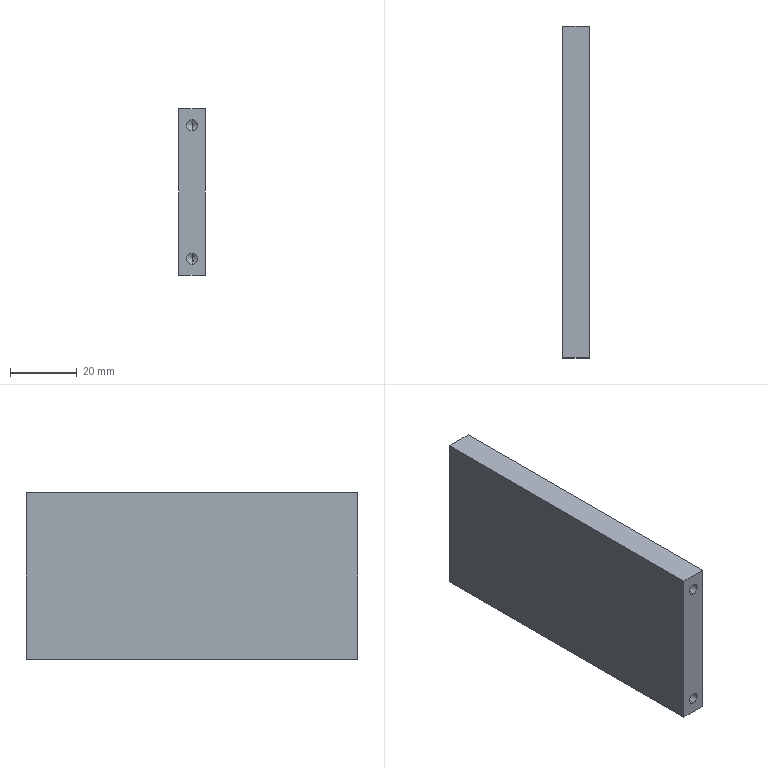Part | STEP file | 0243_211_Plate | 1 solid | 22 faces | box 8 x 99.5 x 50 mm | volume 39443 mm3 | cylinder 8 | cone 8 | plane 6 | commonest cylinder face diameters 3.3 x8